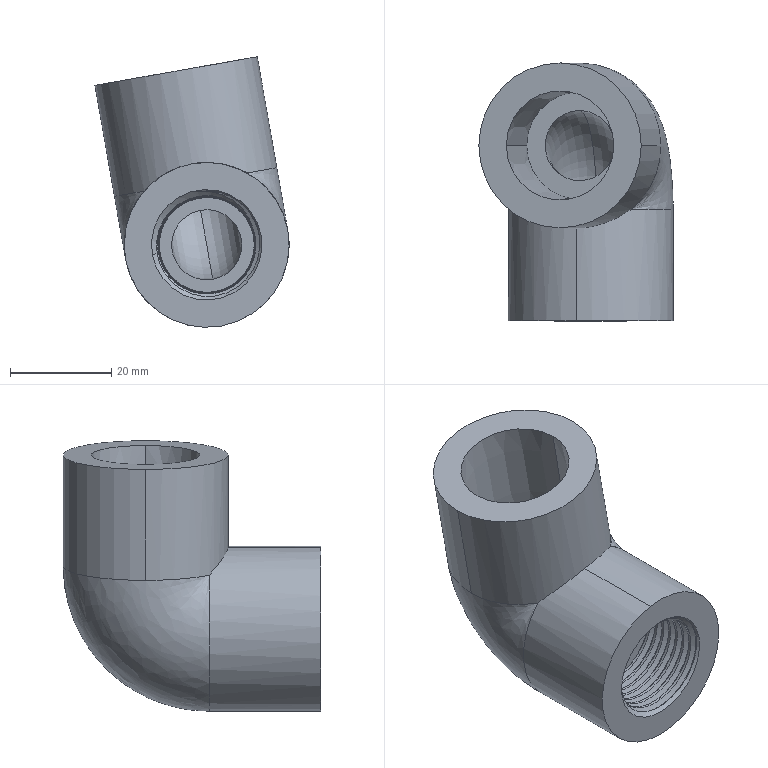Part | SolidWorks | 1 solid | 36 faces | box 38.308 x 50.8 x 53.348 mm | volume 36744 mm3 | cone 20 | cylinder 6 | spline 4 | plane 4 | torus 2 | commonest cylinder face diameters 32.512 x4 13.868 x2